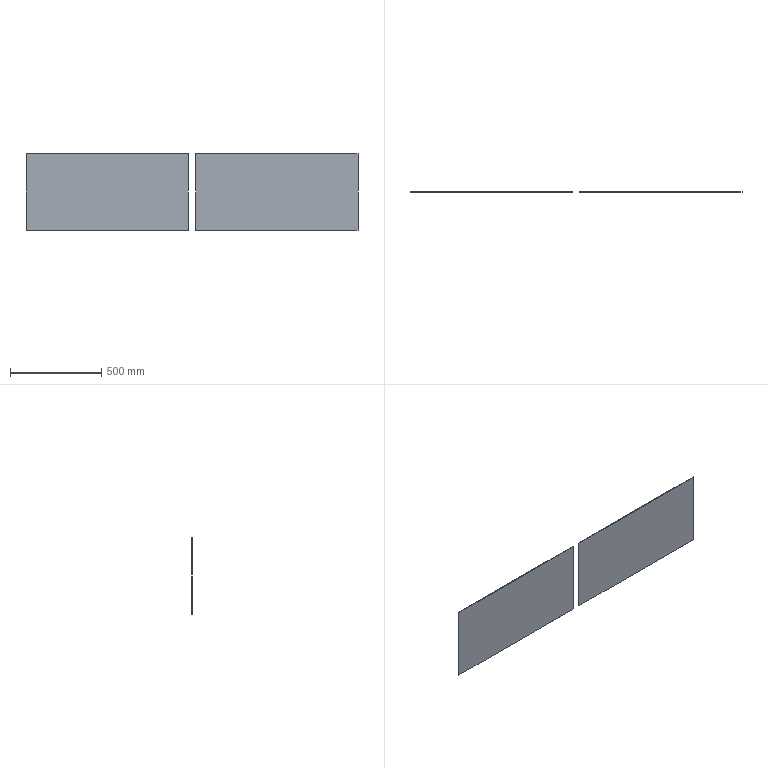Part | SolidWorks | features ICE 5, Extrusion 1 | 2 solids | 12 faces | box 1822 x 4 x 420 mm | volume 2993760 mm3 | plane 12
STEP:
#1=CARTESIAN_POINT('',(911.,0.,-210.));
#2=VERTEX_POINT('',#1);
#3=CARTESIAN_POINT('',(20.,0.,-210.));
#4=VERTEX_POINT('',#3);
#5=CARTESIAN_POINT('',(-911.,0.,-210.));
#6=DIRECTION('',(-1.,0.,0.));
#7=VECTOR('',#6,1000.);
#8=LINE('',#5,#7);
#9=EDGE_CURVE('',#2,#4,#8,.T.);
#10=ORIENTED_EDGE('',*,*,#9,.T.);
#11=CARTESIAN_POINT('',(20.,4.,-210.));
#12=VERTEX_POINT('',#11);
#13=CARTESIAN_POINT('',(20.,4.,-210.));
#14=DIRECTION('',(0.,1.,0.));
#15=VECTOR('',#14,1000.);
#16=LINE('',#13,#15);
#17=EDGE_CURVE('',#4,#12,#16,.T.);
#18=ORIENTED_EDGE('',*,*,#17,.T.);
#19=CARTESIAN_POINT('',(911.,4.,-210.));
#20=VERTEX_POINT('',#19);
#21=CARTESIAN_POINT('',(-911.,4.,-210.));
#22=DIRECTION('',(-1.,0.,0.));
#23=VECTOR('',#22,1000.);
#24=LINE('',#21,#23);
#25=EDGE_CURVE('',#20,#12,#24,.T.);
#26=ORIENTED_EDGE('',*,*,#25,.F.);
#27=CARTESIAN_POINT('',(911.,4.,-210.));
#28=DIRECTION('',(0.,-1.,0.));
#29=VECTOR('',#28,1000.);
#30=LINE('',#27,#29);
#31=EDGE_CURVE('',#20,#2,#30,.T.);
#32=ORIENTED_EDGE('',*,*,#31,.T.);
#33=EDGE_LOOP('',(#10,#18,#26,#32));
#34=FACE_OUTER_BOUND('',#33,.T.);
#35=CARTESIAN_POINT('',(-911.,4.,-210.));
#36=DIRECTION('',(0.,0.,1.));
#37=DIRECTION('',(1.,0.,0.));
#38=AXIS2_PLACEMENT_3D('',#35,#36,#37);
#39=PLANE('',#38);
#40=ADVANCED_FACE('',(#34),#39,.F.);
#41=CARTESIAN_POINT('',(20.,4.,210.));
#42=VERTEX_POINT('',#41);
#43=CARTESIAN_POINT('',(911.,4.,210.));
#44=VERTEX_POINT('',#43);
#45=CARTESIAN_POINT('',(-911.,4.,210.));
#46=DIRECTION('',(1.,0.,0.));
#47=VECTOR('',#46,1000.);
#48=LINE('',#45,#47);
#49=EDGE_CURVE('',#42,#44,#48,.T.);
#50=ORIENTED_EDGE('',*,*,#49,.F.);
#51=CARTESIAN_POINT('',(20.,0.,210.));
#52=VERTEX_POINT('',#51);
#53=CARTESIAN_POINT('',(20.,4.,210.));
#54=DIRECTION('',(0.,-1.,0.));
#55=VECTOR('',#54,1000.);
#56=LINE('',#53,#55);
#57=EDGE_CURVE('',#42,#52,#56,.T.);
#58=ORIENTED_EDGE('',*,*,#57,.T.);
#59=CARTESIAN_POINT('',(911.,0.,210.));
#60=VERTEX_POINT('',#59);
#61=CARTESIAN_POINT('',(-911.,0.,210.));
#62=DIRECTION('',(1.,0.,0.));
#63=VECTOR('',#62,1000.);
#64=LINE('',#61,#63);
#65=EDGE_CURVE('',#52,#60,#64,.T.);
#66=ORIENTED_EDGE('',*,*,#65,.T.);
#67=CARTESIAN_POINT('',(911.,4.,210.));
#68=DIRECTION('',(0.,-1.,0.));
#69=VECTOR('',#68,1000.);
#70=LINE('',#67,#69);
#71=EDGE_CURVE('',#44,#60,#70,.T.);
#72=ORIENTED_EDGE('',*,*,#71,.F.);
#73=EDGE_LOOP('',(#50,#58,#66,#72));
#74=FACE_OUTER_BOUND('',#73,.T.);
#75=CARTESIAN_POINT('',(-911.,4.,210.));
#76=DIRECTION('',(0.,0.,-1.));
#77=DIRECTION('',(-1.,0.,0.));
#78=AXIS2_PLACEMENT_3D('',#75,#76,#77);
#79=PLANE('',#78);
#80=ADVANCED_FACE('',(#74),#79,.F.);
#81=CARTESIAN_POINT('',(20.,4.,-286.888));
#82=DIRECTION('',(0.,0.,-1.));
#83=VECTOR('',#82,1000.);
#84=LINE('',#81,#83);
#85=EDGE_CURVE('',#42,#12,#84,.T.);
#86=ORIENTED_EDGE('',*,*,#85,.F.);
#87=ORIENTED_EDGE('',*,*,#49,.T.);
#88=CARTESIAN_POINT('',(911.,4.,-210.));
#89=DIRECTION('',(0.,0.,-1.));
#90=VECTOR('',#89,1000.);
#91=LINE('',#88,#90);
#92=EDGE_CURVE('',#44,#20,#91,.T.);
#93=ORIENTED_EDGE('',*,*,#92,.T.);
#94=ORIENTED_EDGE('',*,*,#25,.T.);
#95=EDGE_LOOP('',(#86,#87,#93,#94));
#96=FACE_OUTER_BOUND('',#95,.T.);
#97=CARTESIAN_POINT('',(0.,4.,0.));
#98=DIRECTION('',(0.,1.,0.));
#99=DIRECTION('',(0.,0.,1.));
#100=AXIS2_PLACEMENT_3D('',#97,#98,#99);
#101=PLANE('',#100);
#102=ADVANCED_FACE('',(#96),#101,.T.);
#103=ORIENTED_EDGE('',*,*,#65,.F.);
#104=CARTESIAN_POINT('',(20.,0.,0.));
#105=DIRECTION('',(0.,0.,-1.));
#106=VECTOR('',#105,1000.);
#107=LINE('',#104,#106);
#108=EDGE_CURVE('',#52,#4,#107,.T.);
#109=ORIENTED_EDGE('',*,*,#108,.T.);
#110=ORIENTED_EDGE('',*,*,#9,.F.);
#111=CARTESIAN_POINT('',(911.,0.,-210.));
#112=DIRECTION('',(0.,0.,-1.));
#113=VECTOR('',#112,1000.);
#114=LINE('',#111,#113);
#115=EDGE_CURVE('',#60,#2,#114,.T.);
#116=ORIENTED_EDGE('',*,*,#115,.F.);
#117=EDGE_LOOP('',(#103,#109,#110,#116));
#118=FACE_OUTER_BOUND('',#117,.T.);
#119=CARTESIAN_POINT('',(0.,0.,0.));
#120=DIRECTION('',(0.,1.,0.));
#121=DIRECTION('',(0.,0.,1.));
#122=AXIS2_PLACEMENT_3D('',#119,#120,#121);
#123=PLANE('',#122);
#124=ADVANCED_FACE('',(#118),#123,.F.);
#125=ORIENTED_EDGE('',*,*,#115,.T.);
#126=ORIENTED_EDGE('',*,*,#31,.F.);
#127=ORIENTED_EDGE('',*,*,#92,.F.);
#128=ORIENTED_EDGE('',*,*,#71,.T.);
#129=EDGE_LOOP('',(#125,#126,#127,#128));
#130=FACE_OUTER_BOUND('',#129,.T.);
#131=CARTESIAN_POINT('',(911.,4.,-210.));
#132=DIRECTION('',(-1.,0.,0.));
#133=DIRECTION('',(0.,0.,1.));
#134=AXIS2_PLACEMENT_3D('',#131,#132,#133);
#135=PLANE('',#134);
#136=ADVANCED_FACE('',(#130),#135,.F.);
#137=ORIENTED_EDGE('',*,*,#108,.F.);
#138=ORIENTED_EDGE('',*,*,#57,.F.);
#139=ORIENTED_EDGE('',*,*,#85,.T.);
#140=ORIENTED_EDGE('',*,*,#17,.F.);
#141=EDGE_LOOP('',(#137,#138,#139,#140));
#142=FACE_OUTER_BOUND('',#141,.T.);
#143=CARTESIAN_POINT('',(20.,0.,-286.888));
#144=DIRECTION('',(1.,0.,0.));
#145=DIRECTION('',(0.,0.,-1.));
#146=AXIS2_PLACEMENT_3D('',#143,#144,#145);
#147=PLANE('',#146);
#148=ADVANCED_FACE('',(#142),#147,.F.);
#149=CLOSED_SHELL('',(#40,#80,#102,#124,#136,#148));
#150=MANIFOLD_SOLID_BREP('',#149);
#151=CARTESIAN_POINT('',(-911.,0.,-210.));
#152=VERTEX_POINT('',#151);
#153=CARTESIAN_POINT('',(-911.,0.,210.));
#154=VERTEX_POINT('',#153);
#155=CARTESIAN_POINT('',(-911.,0.,-210.));
#156=DIRECTION('',(0.,0.,1.));
#157=VECTOR('',#156,1000.);
#158=LINE('',#155,#157);
#159=EDGE_CURVE('',#152,#154,#158,.T.);
#160=ORIENTED_EDGE('',*,*,#159,.T.);
#161=CARTESIAN_POINT('',(-911.,4.,210.));
#162=VERTEX_POINT('',#161);
#163=CARTESIAN_POINT('',(-911.,4.,210.));
#164=DIRECTION('',(0.,-1.,0.));
#165=VECTOR('',#164,1000.);
#166=LINE('',#163,#165);
#167=EDGE_CURVE('',#162,#154,#166,.T.);
#168=ORIENTED_EDGE('',*,*,#167,.F.);
#169=CARTESIAN_POINT('',(-911.,4.,-210.));
#170=VERTEX_POINT('',#169);
#171=CARTESIAN_POINT('',(-911.,4.,-210.));
#172=DIRECTION('',(0.,0.,1.));
#173=VECTOR('',#172,1000.);
#174=LINE('',#171,#173);
#175=EDGE_CURVE('',#170,#162,#174,.T.);
#176=ORIENTED_EDGE('',*,*,#175,.F.);
#177=CARTESIAN_POINT('',(-911.,4.,-210.));
#178=DIRECTION('',(0.,-1.,0.));
#179=VECTOR('',#178,1000.);
#180=LINE('',#177,#179);
#181=EDGE_CURVE('',#170,#152,#180,.T.);
#182=ORIENTED_EDGE('',*,*,#181,.T.);
#183=EDGE_LOOP('',(#160,#168,#176,#182));
#184=FACE_OUTER_BOUND('',#183,.T.);
#185=CARTESIAN_POINT('',(-911.,4.,-210.));
#186=DIRECTION('',(1.,0.,0.));
#187=DIRECTION('',(0.,0.,-1.));
#188=AXIS2_PLACEMENT_3D('',#185,#186,#187);
#189=PLANE('',#188);
#190=ADVANCED_FACE('',(#184),#189,.F.);
#191=CARTESIAN_POINT('',(-20.,4.,-210.));
#192=VERTEX_POINT('',#191);
#193=CARTESIAN_POINT('',(-20.,4.,210.));
#194=VERTEX_POINT('',#193);
#195=CARTESIAN_POINT('',(-20.,4.,-286.888));
#196=DIRECTION('',(0.,0.,1.));
#197=VECTOR('',#196,1000.);
#198=LINE('',#195,#197);
#199=EDGE_CURVE('',#192,#194,#198,.T.);
#200=ORIENTED_EDGE('',*,*,#199,.F.);
#201=CARTESIAN_POINT('',(-911.,4.,-210.));
#202=DIRECTION('',(-1.,0.,0.));
#203=VECTOR('',#202,1000.);
#204=LINE('',#201,#203);
#205=EDGE_CURVE('',#192,#170,#204,.T.);
#206=ORIENTED_EDGE('',*,*,#205,.T.);
#207=ORIENTED_EDGE('',*,*,#175,.T.);
#208=CARTESIAN_POINT('',(-911.,4.,210.));
#209=DIRECTION('',(1.,0.,0.));
#210=VECTOR('',#209,1000.);
#211=LINE('',#208,#210);
#212=EDGE_CURVE('',#162,#194,#211,.T.);
#213=ORIENTED_EDGE('',*,*,#212,.T.);
#214=EDGE_LOOP('',(#200,#206,#207,#213));
#215=FACE_OUTER_BOUND('',#214,.T.);
#216=CARTESIAN_POINT('',(0.,4.,0.));
#217=DIRECTION('',(0.,1.,0.));
#218=DIRECTION('',(0.,0.,1.));
#219=AXIS2_PLACEMENT_3D('',#216,#217,#218);
#220=PLANE('',#219);
#221=ADVANCED_FACE('',(#215),#220,.T.);
#222=CARTESIAN_POINT('',(-20.,0.,-210.));
#223=VERTEX_POINT('',#222);
#224=CARTESIAN_POINT('',(-911.,0.,-210.));
#225=DIRECTION('',(-1.,0.,0.));
#226=VECTOR('',#225,1000.);
#227=LINE('',#224,#226);
#228=EDGE_CURVE('',#223,#152,#227,.T.);
#229=ORIENTED_EDGE('',*,*,#228,.F.);
#230=CARTESIAN_POINT('',(-20.,0.,210.));
#231=VERTEX_POINT('',#230);
#232=CARTESIAN_POINT('',(-20.,0.,0.));
#233=DIRECTION('',(0.,0.,1.));
#234=VECTOR('',#233,1000.);
#235=LINE('',#232,#234);
#236=EDGE_CURVE('',#223,#231,#235,.T.);
#237=ORIENTED_EDGE('',*,*,#236,.T.);
#238=CARTESIAN_POINT('',(-911.,0.,210.));
#239=DIRECTION('',(1.,0.,0.));
#240=VECTOR('',#239,1000.);
#241=LINE('',#238,#240);
#242=EDGE_CURVE('',#154,#231,#241,.T.);
#243=ORIENTED_EDGE('',*,*,#242,.F.);
#244=ORIENTED_EDGE('',*,*,#159,.F.);
#245=EDGE_LOOP('',(#229,#237,#243,#244));
#246=FACE_OUTER_BOUND('',#245,.T.);
#247=CARTESIAN_POINT('',(0.,0.,0.));
#248=DIRECTION('',(0.,1.,0.));
#249=DIRECTION('',(0.,0.,1.));
#250=AXIS2_PLACEMENT_3D('',#247,#248,#249);
#251=PLANE('',#250);
#252=ADVANCED_FACE('',(#246),#251,.F.);
#253=ORIENTED_EDGE('',*,*,#242,.T.);
#254=CARTESIAN_POINT('',(-20.,4.,210.));
#255=DIRECTION('',(0.,1.,0.));
#256=VECTOR('',#255,1000.);
#257=LINE('',#254,#256);
#258=EDGE_CURVE('',#231,#194,#257,.T.);
#259=ORIENTED_EDGE('',*,*,#258,.T.);
#260=ORIENTED_EDGE('',*,*,#212,.F.);
#261=ORIENTED_EDGE('',*,*,#167,.T.);
#262=EDGE_LOOP('',(#253,#259,#260,#261));
#263=FACE_OUTER_BOUND('',#262,.T.);
#264=CARTESIAN_POINT('',(-911.,4.,210.));
#265=DIRECTION('',(0.,0.,-1.));
#266=DIRECTION('',(-1.,0.,0.));
#267=AXIS2_PLACEMENT_3D('',#264,#265,#266);
#268=PLANE('',#267);
#269=ADVANCED_FACE('',(#263),#268,.F.);
#270=ORIENTED_EDGE('',*,*,#205,.F.);
#271=CARTESIAN_POINT('',(-20.,4.,-210.));
#272=DIRECTION('',(0.,-1.,0.));
#273=VECTOR('',#272,1000.);
#274=LINE('',#271,#273);
#275=EDGE_CURVE('',#192,#223,#274,.T.);
#276=ORIENTED_EDGE('',*,*,#275,.T.);
#277=ORIENTED_EDGE('',*,*,#228,.T.);
#278=ORIENTED_EDGE('',*,*,#181,.F.);
#279=EDGE_LOOP('',(#270,#276,#277,#278));
#280=FACE_OUTER_BOUND('',#279,.T.);
#281=CARTESIAN_POINT('',(-911.,4.,-210.));
#282=DIRECTION('',(0.,0.,1.));
#283=DIRECTION('',(1.,0.,0.));
#284=AXIS2_PLACEMENT_3D('',#281,#282,#283);
#285=PLANE('',#284);
#286=ADVANCED_FACE('',(#280),#285,.F.);
#287=ORIENTED_EDGE('',*,*,#199,.T.);
#288=ORIENTED_EDGE('',*,*,#258,.F.);
#289=ORIENTED_EDGE('',*,*,#236,.F.);
#290=ORIENTED_EDGE('',*,*,#275,.F.);
#291=EDGE_LOOP('',(#287,#288,#289,#290));
#292=FACE_OUTER_BOUND('',#291,.T.);
#293=CARTESIAN_POINT('',(-20.,0.,-286.888));
#294=DIRECTION('',(-1.,0.,0.));
#295=DIRECTION('',(0.,0.,1.));
#296=AXIS2_PLACEMENT_3D('',#293,#294,#295);
#297=PLANE('',#296);
#298=ADVANCED_FACE('',(#292),#297,.F.);
#299=CLOSED_SHELL('',(#190,#221,#252,#269,#286,#298));
#300=MANIFOLD_SOLID_BREP('',#299);
#301=CARTESIAN_POINT('',(0.,0.,0.));
#302=DIRECTION('',(0.,0.,1.));
#303=DIRECTION('',(1.,0.,0.));
#304=AXIS2_PLACEMENT_3D('',#301,#302,#303);
#305=(LENGTH_UNIT()NAMED_UNIT(*)SI_UNIT(.MILLI.,.METRE.));
#306=UNCERTAINTY_MEASURE_WITH_UNIT(LENGTH_MEASURE(0.00001),#305,'','');
#307=(NAMED_UNIT(*)PLANE_ANGLE_UNIT()SI_UNIT($,.RADIAN.));
#308=(NAMED_UNIT(*)SI_UNIT($,.STERADIAN.)SOLID_ANGLE_UNIT());
#309=(GEOMETRIC_REPRESENTATION_CONTEXT(3)GLOBAL_UNCERTAINTY_ASSIGNED_CONTEXT((#306))GLOBAL_UNIT_ASSIGNED_CONTEXT((#305,#307,#308))REPRESENTATION_CONTEXT('',''));
#310=ADVANCED_BREP_SHAPE_REPRESENTATION('',(#150,#300,#304),#309);